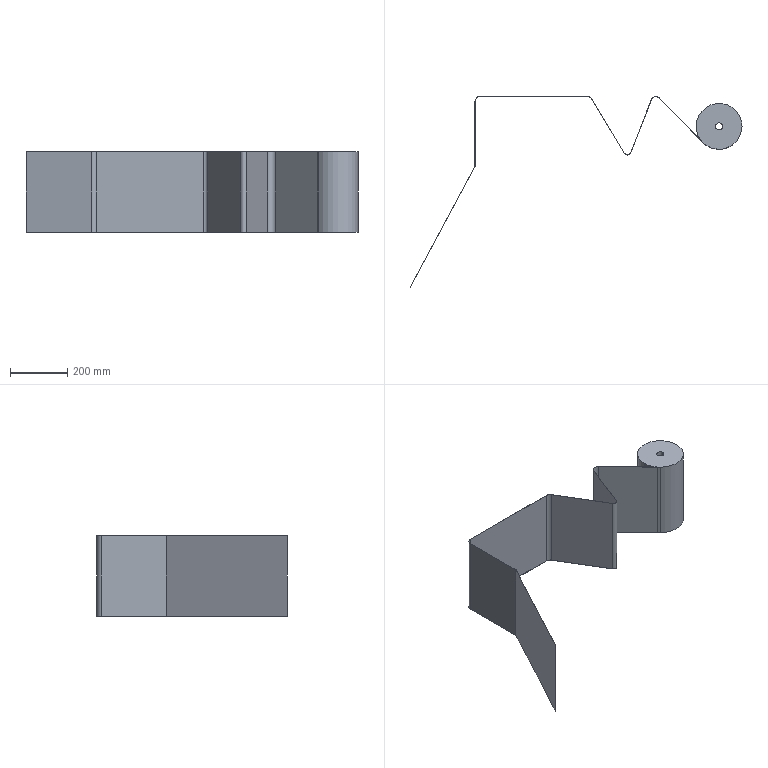Part | STEP file | 1 solid | 28 faces | box 1160 x 667.187 x 280 mm | volume 5746946 mm3 | plane 15 | cylinder 13 | commonest cylinder face diameters 25 x3 36 x3 37 x3 160 x3 24 x1